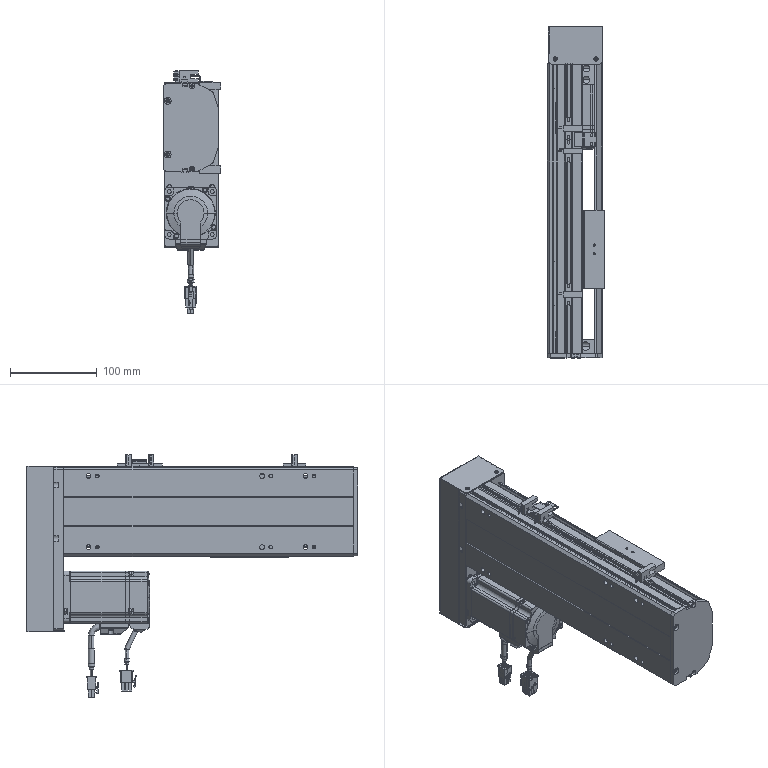Part | SolidWorks | features CompositeCurve 1 | 20 solids | 1881 faces | box 66 x 382.5 x 279.882 mm | volume 1255947 mm3 | plane 1067 | cylinder 625 | cone 151 | spline 34 | torus 4 | commonest cylinder face diameters 1 x55 5.5 x44 8 x41 4 x39 6 x35 10 x34